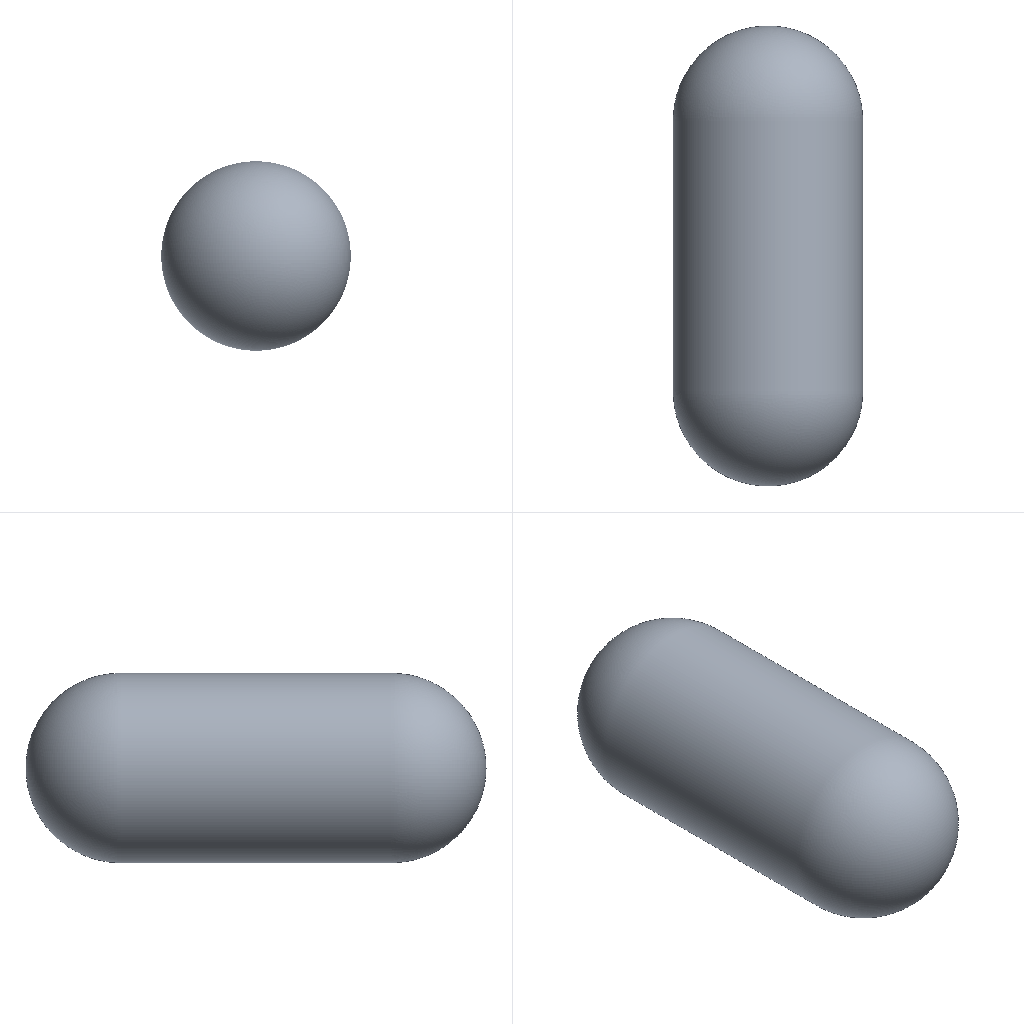Simulation study | abaqus
Set-up summary:
category,name,step,type,value,unit,region
solver,abaqus
solver,version,,,Abaqus/Standard 3DEXPERIENCE R2017x
units,not stated in the deck,,not stated
analysis,deck,,coupled temperature-displacement,coupled temperature-displacement
load_step,Step-1,Step-1,coupled temperature-displacement,nlgeom=True
contact,interactions,,,general=0 pairs=0 ties=0
load_step,requested,,,1
mesh,nodes,,,50516
mesh,elements,,,25256
element_type,C3D8RT,,solid,25256
load,load commands in deck,,count,1
bc,support commands in deck,,count,1
material,MATERIAL-1,,in results
check,setup vs results,,match,"per instance, exact: element labels, types and connectivity; labels of the nodes the elements use; coordinates of those nodes at SINGLE_PRECISION in 1 of 1 instance(s)"
Abaqus input file, long lists of numbers shortened:
*Heading
** Job name: Job-2 Model name: Model-1-Copy
** Generated by: Abaqus/CAE 2017
*Preprint, echo=NO, model=NO, history=NO, contact=NO
**
** PARTS
**
*Part, name=Part-1
*Node
      1,        -400.,         450.,           0.
      2,         400.,         450.,           0.
** (50514 more lines like these left out)
*Element, type=C3D8RT
   1,   518,  1361,  8234,   361,     1,    13,   186,     4
   2,  1361,  1362,  8235,  8234,    13,    14,   185,   186
** (25254 more lines like these left out)
*Nset, nset=Set-2, generate
     1,  50516,      1
*Elset, elset=Set-2, generate
     1,  25256,      1
** Section: Section-1
*Solid Section, elset=Set-2, material=Material-1
,
*End Part
**
**
** ASSEMBLY
**
*Assembly, name=Assembly
**
*Instance, name=Part-1-1, part=Part-1
       -420.,         720.,           0.
*End Instance
**
*Nset, nset=Set-1, instance=Part-1-1, generate
     1,  50516,      1
*Elset, elset=Set-1, instance=Part-1-1, generate
     1,  25256,      1
*Nset, nset=Set-2, instance=Part-1-1
 10, 11
*End Assembly
**
** MATERIALS
**
*Material, name=Material-1
*Conductivity
46.,
*Density
 7.8e-09,
*Elastic
210000., 0.3
*Expansion
 1e-05,
*Plastic
310.,   0.
420., 0.01
*Specific Heat
 6.7e+08,
** ----------------------------------------------------------------
**
** STEP: Step-1
**
*Step, name=Step-1, nlgeom=YES, inc=1000
*Coupled Temperature-displacement, creep=none, deltmx=100000., stabilize=0.0002, allsdtol=0.05, continue=NO
0.1, 10., 0.0001, 0.2
**
** BOUNDARY CONDITIONS
**
** Name: BC-1 Type: 对称/反对称/完全固定
*Boundary
Set-2, ENCASTRE
**
** LOADS
**
** Name: Load-1   Type: Body heat flux
*Dflux
Set-1, BFNU, 1.
**
** OUTPUT REQUESTS
**
*Restart, write, frequency=0
**
** FIELD OUTPUT: F-Output-1
**
*Output, field
*Node Output
CF, NT, RF, RFL, RM, RT, TF, U
V
*Element Output, directions=YES
ALPHAN, CTSHR, E, HFL, LE, MISES, MISESMAX, MISESONLY, PE, PEEQ, PEEQMAX, PEEQT, PEMAG, PRESSONLY, PS, S
SF, SSAVG, TEMP, TSHR
*Contact Output
CDISP, CSTRESS
*Radiation Output
FTEMP,
**
** HISTORY OUTPUT: H-Output-1
**
*Output, history, variable=PRESELECT
*End Step
Results summary:
result,step,,completed,increments=52 time=10.0/10.0
result,analysis,,,"coupled temperature-displacement, steady state"
result,last_loadstep,,,1
result,analysis steps,,count,1
result,primary field,,,"U, NT11"
result,reaction total,,FX,-2.9e-05,model units
result,reaction total,,FY,-1.4e-05,model units
result,reaction total,,FZ,-0.0,model units